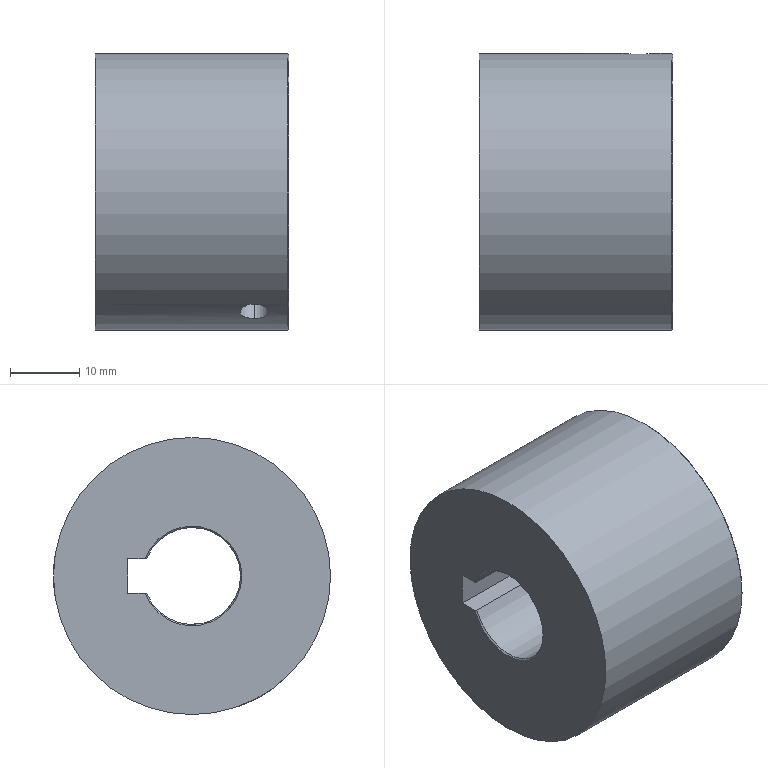Part | STEP file | ATP40XL050-B-N14 | 1 solid | 18 faces | box 28 x 40 x 40 mm | volume 30210 mm3 | cylinder 7 | cone 6 | plane 5 | commonest cylinder face diameters 4.134 x4 14 x2 40 x1
STEP:
#1=CARTESIAN_POINT('',(0.,9.3,2.5));
#2=VERTEX_POINT('',#1);
#3=CARTESIAN_POINT('',(0.,6.752,2.5));
#4=VERTEX_POINT('',#3);
#5=CARTESIAN_POINT('',(0.,9.,2.5));
#6=DIRECTION('',(0.,-1.,0.));
#7=VECTOR('',#6,1000.);
#8=LINE('',#5,#7);
#9=EDGE_CURVE('',#2,#4,#8,.T.);
#10=ORIENTED_EDGE('',*,*,#9,.T.);
#11=CARTESIAN_POINT('',(0.,-7.2,0.));
#12=VERTEX_POINT('',#11);
#13=CARTESIAN_POINT('',(0.,0.,0.));
#14=DIRECTION('',(-1.,0.,0.));
#15=DIRECTION('',(0.,1.,0.));
#16=AXIS2_PLACEMENT_3D('',#13,#14,#15);
#17=CIRCLE('',#16,7.2);
#18=EDGE_CURVE('',#12,#4,#17,.T.);
#19=ORIENTED_EDGE('',*,*,#18,.F.);
#20=CARTESIAN_POINT('',(0.,6.752,-2.5));
#21=VERTEX_POINT('',#20);
#22=CARTESIAN_POINT('',(0.,0.,0.));
#23=DIRECTION('',(-1.,0.,0.));
#24=DIRECTION('',(0.,1.,0.));
#25=AXIS2_PLACEMENT_3D('',#22,#23,#24);
#26=CIRCLE('',#25,7.2);
#27=EDGE_CURVE('',#21,#12,#26,.T.);
#28=ORIENTED_EDGE('',*,*,#27,.F.);
#29=CARTESIAN_POINT('',(0.,9.3,-2.5));
#30=VERTEX_POINT('',#29);
#31=CARTESIAN_POINT('',(0.,13.65,-2.5));
#32=DIRECTION('',(0.,1.,0.));
#33=VECTOR('',#32,1000.);
#34=LINE('',#31,#33);
#35=EDGE_CURVE('',#21,#30,#34,.T.);
#36=ORIENTED_EDGE('',*,*,#35,.T.);
#37=CARTESIAN_POINT('',(0.,9.3,1.25));
#38=DIRECTION('',(0.,0.,1.));
#39=VECTOR('',#38,1000.);
#40=LINE('',#37,#39);
#41=EDGE_CURVE('',#30,#2,#40,.T.);
#42=ORIENTED_EDGE('',*,*,#41,.T.);
#43=EDGE_LOOP('',(#10,#19,#28,#36,#42));
#44=FACE_BOUND('',#43,.T.);
#45=CARTESIAN_POINT('',(0.,0.,20.));
#46=VERTEX_POINT('',#45);
#47=CARTESIAN_POINT('',(0.,0.,0.));
#48=DIRECTION('',(-1.,0.,0.));
#49=DIRECTION('',(0.,0.,1.));
#50=AXIS2_PLACEMENT_3D('',#47,#48,#49);
#51=CIRCLE('',#50,20.);
#52=EDGE_CURVE('',#46,#46,#51,.T.);
#53=ORIENTED_EDGE('',*,*,#52,.T.);
#54=EDGE_LOOP('',(#53));
#55=FACE_OUTER_BOUND('',#54,.T.);
#56=CARTESIAN_POINT('',(0.,18.,0.));
#57=DIRECTION('',(-1.,0.,0.));
#58=DIRECTION('',(0.,0.,1.));
#59=AXIS2_PLACEMENT_3D('',#56,#57,#58);
#60=PLANE('',#59);
#61=ADVANCED_FACE('',(#44,#55),#60,.T.);
#62=CARTESIAN_POINT('',(28.,19.8,0.));
#63=VERTEX_POINT('',#62);
#64=CARTESIAN_POINT('',(27.8,20.,0.));
#65=VERTEX_POINT('',#64);
#66=CARTESIAN_POINT('',(27.9,19.9,0.));
#67=DIRECTION('',(-0.7071,0.7071,0.));
#68=VECTOR('',#67,1000.);
#69=LINE('',#66,#68);
#70=EDGE_CURVE('',#63,#65,#69,.T.);
#71=ORIENTED_EDGE('',*,*,#70,.F.);
#72=CARTESIAN_POINT('',(28.,-19.8,0.));
#73=VERTEX_POINT('',#72);
#74=CARTESIAN_POINT('',(28.,0.,0.));
#75=DIRECTION('',(-1.,0.,0.));
#76=DIRECTION('',(0.,1.,0.));
#77=AXIS2_PLACEMENT_3D('',#74,#75,#76);
#78=CIRCLE('',#77,19.8);
#79=EDGE_CURVE('',#63,#73,#78,.T.);
#80=ORIENTED_EDGE('',*,*,#79,.T.);
#81=CARTESIAN_POINT('',(27.8,-20.,0.));
#82=VERTEX_POINT('',#81);
#83=CARTESIAN_POINT('',(27.9,-19.9,0.));
#84=DIRECTION('',(0.7071,0.7071,0.));
#85=VECTOR('',#84,1000.);
#86=LINE('',#83,#85);
#87=EDGE_CURVE('',#82,#73,#86,.T.);
#88=ORIENTED_EDGE('',*,*,#87,.F.);
#89=CARTESIAN_POINT('',(27.8,0.,0.));
#90=DIRECTION('',(-1.,0.,0.));
#91=DIRECTION('',(0.,1.,0.));
#92=AXIS2_PLACEMENT_3D('',#89,#90,#91);
#93=CIRCLE('',#92,20.);
#94=EDGE_CURVE('',#65,#82,#93,.T.);
#95=ORIENTED_EDGE('',*,*,#94,.F.);
#96=EDGE_LOOP('',(#71,#80,#88,#95));
#97=FACE_OUTER_BOUND('',#96,.T.);
#98=CARTESIAN_POINT('',(27.9,0.,0.));
#99=DIRECTION('',(-1.,0.,0.));
#100=DIRECTION('',(0.,1.,0.));
#101=AXIS2_PLACEMENT_3D('',#98,#99,#100);
#102=CONICAL_SURFACE('',#101,19.9,0.7854);
#103=ADVANCED_FACE('',(#97),#102,.T.);
#104=CARTESIAN_POINT('',(0.2,-7.,0.));
#105=VERTEX_POINT('',#104);
#106=CARTESIAN_POINT('',(27.8,-7.,0.));
#107=VERTEX_POINT('',#106);
#108=CARTESIAN_POINT('',(14.,-7.,0.));
#109=DIRECTION('',(1.,0.,0.));
#110=VECTOR('',#109,1000.);
#111=LINE('',#108,#110);
#112=EDGE_CURVE('',#105,#107,#111,.T.);
#113=ORIENTED_EDGE('',*,*,#112,.F.);
#114=CARTESIAN_POINT('',(0.2,6.538,2.5));
#115=VERTEX_POINT('',#114);
#116=CARTESIAN_POINT('',(0.2,0.,0.));
#117=DIRECTION('',(-1.,0.,0.));
#118=DIRECTION('',(0.,1.,0.));
#119=AXIS2_PLACEMENT_3D('',#116,#117,#118);
#120=CIRCLE('',#119,7.);
#121=EDGE_CURVE('',#105,#115,#120,.T.);
#122=ORIENTED_EDGE('',*,*,#121,.T.);
#123=CARTESIAN_POINT('',(27.8,6.538,2.5));
#124=VERTEX_POINT('',#123);
#125=CARTESIAN_POINT('',(14.,6.538,2.5));
#126=DIRECTION('',(1.,0.,0.));
#127=VECTOR('',#126,1000.);
#128=LINE('',#125,#127);
#129=EDGE_CURVE('',#115,#124,#128,.T.);
#130=ORIENTED_EDGE('',*,*,#129,.T.);
#131=CARTESIAN_POINT('',(27.8,0.,0.));
#132=DIRECTION('',(-1.,0.,0.));
#133=DIRECTION('',(0.,1.,0.));
#134=AXIS2_PLACEMENT_3D('',#131,#132,#133);
#135=CIRCLE('',#134,7.);
#136=EDGE_CURVE('',#107,#124,#135,.T.);
#137=ORIENTED_EDGE('',*,*,#136,.F.);
#138=EDGE_LOOP('',(#113,#122,#130,#137));
#139=FACE_OUTER_BOUND('',#138,.T.);
#140=CARTESIAN_POINT('',(14.,0.,0.));
#141=DIRECTION('',(1.,0.,0.));
#142=DIRECTION('',(0.,1.,0.));
#143=AXIS2_PLACEMENT_3D('',#140,#141,#142);
#144=CYLINDRICAL_SURFACE('',#143,7.);
#145=ADVANCED_FACE('',(#139),#144,.F.);
#146=CARTESIAN_POINT('',(0.1,-7.1,0.));
#147=DIRECTION('',(0.7071,0.7071,0.));
#148=VECTOR('',#147,1000.);
#149=LINE('',#146,#148);
#150=EDGE_CURVE('',#12,#105,#149,.T.);
#151=ORIENTED_EDGE('',*,*,#150,.F.);
#152=ORIENTED_EDGE('',*,*,#18,.T.);
#153=CARTESIAN_POINT('',(0.,6.752,2.5));
#154=CARTESIAN_POINT('',(0.1016,6.644,2.5));
#155=CARTESIAN_POINT('',(0.2,6.538,2.5));
#156=(BOUNDED_CURVE()B_SPLINE_CURVE(2,(#153,#154,#155),.UNSPECIFIED.,.F.,.F.)B_SPLINE_CURVE_WITH_KNOTS((3,3),(0.,0.2927),.UNSPECIFIED.)CURVE()GEOMETRIC_REPRESENTATION_ITEM()RATIONAL_B_SPLINE_CURVE((1.,1.,1.))REPRESENTATION_ITEM(''));
#157=EDGE_CURVE('',#4,#115,#156,.T.);
#158=ORIENTED_EDGE('',*,*,#157,.T.);
#159=ORIENTED_EDGE('',*,*,#121,.F.);
#160=EDGE_LOOP('',(#151,#152,#158,#159));
#161=FACE_OUTER_BOUND('',#160,.T.);
#162=CARTESIAN_POINT('',(0.1,0.,0.));
#163=DIRECTION('',(-1.,0.,0.));
#164=DIRECTION('',(0.,1.,0.));
#165=AXIS2_PLACEMENT_3D('',#162,#163,#164);
#166=CONICAL_SURFACE('',#165,7.1,0.7854);
#167=ADVANCED_FACE('',(#161),#166,.F.);
#168=CARTESIAN_POINT('',(28.,-7.2,0.));
#169=VERTEX_POINT('',#168);
#170=CARTESIAN_POINT('',(27.9,-7.1,0.));
#171=DIRECTION('',(0.7071,-0.7071,0.));
#172=VECTOR('',#171,1000.);
#173=LINE('',#170,#172);
#174=EDGE_CURVE('',#107,#169,#173,.T.);
#175=ORIENTED_EDGE('',*,*,#174,.F.);
#176=ORIENTED_EDGE('',*,*,#136,.T.);
#177=CARTESIAN_POINT('',(28.,6.752,2.5));
#178=VERTEX_POINT('',#177);
#179=CARTESIAN_POINT('',(27.8,6.538,2.5));
#180=CARTESIAN_POINT('',(27.898,6.644,2.5));
#181=CARTESIAN_POINT('',(28.,6.752,2.5));
#182=(BOUNDED_CURVE()B_SPLINE_CURVE(2,(#179,#180,#181),.UNSPECIFIED.,.F.,.T.)B_SPLINE_CURVE_WITH_KNOTS((3,3),(0.,0.2927),.UNSPECIFIED.)CURVE()GEOMETRIC_REPRESENTATION_ITEM()RATIONAL_B_SPLINE_CURVE((1.,1.,1.))REPRESENTATION_ITEM(''));
#183=EDGE_CURVE('',#124,#178,#182,.T.);
#184=ORIENTED_EDGE('',*,*,#183,.T.);
#185=CARTESIAN_POINT('',(28.,0.,0.));
#186=DIRECTION('',(-1.,0.,0.));
#187=DIRECTION('',(0.,1.,0.));
#188=AXIS2_PLACEMENT_3D('',#185,#186,#187);
#189=CIRCLE('',#188,7.2);
#190=EDGE_CURVE('',#169,#178,#189,.T.);
#191=ORIENTED_EDGE('',*,*,#190,.F.);
#192=EDGE_LOOP('',(#175,#176,#184,#191));
#193=FACE_OUTER_BOUND('',#192,.T.);
#194=CARTESIAN_POINT('',(27.9,0.,0.));
#195=DIRECTION('',(1.,0.,0.));
#196=DIRECTION('',(0.,1.,0.));
#197=AXIS2_PLACEMENT_3D('',#194,#195,#196);
#198=CONICAL_SURFACE('',#197,7.1,0.7854);
#199=ADVANCED_FACE('',(#193),#198,.F.);
#200=CARTESIAN_POINT('',(23.,19.893,-2.067));
#201=VERTEX_POINT('',#200);
#202=CARTESIAN_POINT('',(23.,19.893,2.067));
#203=VERTEX_POINT('',#202);
#204=CARTESIAN_POINT('',(23.,19.893,-2.067));
#205=CARTESIAN_POINT('',(23.137,19.893,-2.067));
#206=CARTESIAN_POINT('',(23.271,19.894,-2.054));
#207=CARTESIAN_POINT('',(23.535,19.9,-2.001));
#208=CARTESIAN_POINT('',(23.666,19.904,-1.961));
#209=CARTESIAN_POINT('',(23.916,19.914,-1.858));
#210=CARTESIAN_POINT('',(24.035,19.919,-1.794));
#211=CARTESIAN_POINT('',(24.26,19.932,-1.644));
#212=CARTESIAN_POINT('',(24.366,19.94,-1.557));
#213=CARTESIAN_POINT('',(24.652,19.96,-1.272));
#214=CARTESIAN_POINT('',(24.806,19.974,-1.041));
#215=CARTESIAN_POINT('',(25.012,19.994,-0.5445));
#216=CARTESIAN_POINT('',(25.067,20.,-0.2731));
#217=CARTESIAN_POINT('',(25.067,20.,0.1366));
#218=CARTESIAN_POINT('',(25.054,19.999,0.2709));
#219=CARTESIAN_POINT('',(25.001,19.993,0.535));
#220=CARTESIAN_POINT('',(24.961,19.989,0.6663));
#221=CARTESIAN_POINT('',(24.858,19.979,0.9164));
#222=CARTESIAN_POINT('',(24.794,19.974,1.035));
#223=CARTESIAN_POINT('',(24.644,19.961,1.26));
#224=CARTESIAN_POINT('',(24.557,19.954,1.366));
#225=CARTESIAN_POINT('',(24.272,19.933,1.652));
#226=CARTESIAN_POINT('',(24.041,19.919,1.806));
#227=CARTESIAN_POINT('',(23.545,19.899,2.012));
#228=CARTESIAN_POINT('',(23.273,19.893,2.067));
#229=CARTESIAN_POINT('',(23.,19.893,2.067));
#230=B_SPLINE_CURVE_WITH_KNOTS('',3,(#204,#205,#206,#207,#208,#209,#210,#211,#212,#213,#214,#215,#216,#217,#218,#219,#220,#221,#222,#223,#224,#225,#226,#227,#228,#229),.UNSPECIFIED.,.F.,.F.,(4,2,2,2,2,2,2,2,2,2,2,2,4),(0.,0.0004039,0.0008078,0.001212,0.001616,0.002423,0.003231,0.003635,0.004039,0.004443,0.004847,0.005655,0.006462),.UNSPECIFIED.);
#231=EDGE_CURVE('',#201,#203,#230,.T.);
#232=ORIENTED_EDGE('',*,*,#231,.T.);
#233=CARTESIAN_POINT('',(23.,19.893,2.067));
#234=CARTESIAN_POINT('',(22.863,19.893,2.067));
#235=CARTESIAN_POINT('',(22.729,19.894,2.054));
#236=CARTESIAN_POINT('',(22.465,19.9,2.001));
#237=CARTESIAN_POINT('',(22.334,19.904,1.961));
#238=CARTESIAN_POINT('',(22.084,19.914,1.858));
#239=CARTESIAN_POINT('',(21.965,19.919,1.794));
#240=CARTESIAN_POINT('',(21.74,19.932,1.644));
#241=CARTESIAN_POINT('',(21.634,19.94,1.557));
#242=CARTESIAN_POINT('',(21.348,19.96,1.272));
#243=CARTESIAN_POINT('',(21.194,19.974,1.041));
#244=CARTESIAN_POINT('',(20.988,19.994,0.5445));
#245=CARTESIAN_POINT('',(20.933,20.,0.2731));
#246=CARTESIAN_POINT('',(20.933,20.,-0.1366));
#247=CARTESIAN_POINT('',(20.946,19.999,-0.2709));
#248=CARTESIAN_POINT('',(20.999,19.993,-0.535));
#249=CARTESIAN_POINT('',(21.039,19.989,-0.6663));
#250=CARTESIAN_POINT('',(21.142,19.979,-0.9164));
#251=CARTESIAN_POINT('',(21.206,19.974,-1.035));
#252=CARTESIAN_POINT('',(21.356,19.961,-1.26));
#253=CARTESIAN_POINT('',(21.443,19.954,-1.366));
#254=CARTESIAN_POINT('',(21.728,19.933,-1.652));
#255=CARTESIAN_POINT('',(21.959,19.919,-1.806));
#256=CARTESIAN_POINT('',(22.455,19.899,-2.012));
#257=CARTESIAN_POINT('',(22.727,19.893,-2.067));
#258=CARTESIAN_POINT('',(23.,19.893,-2.067));
#259=B_SPLINE_CURVE_WITH_KNOTS('',3,(#233,#234,#235,#236,#237,#238,#239,#240,#241,#242,#243,#244,#245,#246,#247,#248,#249,#250,#251,#252,#253,#254,#255,#256,#257,#258),.UNSPECIFIED.,.F.,.F.,(4,2,2,2,2,2,2,2,2,2,2,2,4),(-0.003231,-0.002827,-0.002423,-0.002019,-0.001616,-0.0008078,0.000000013,0.0004039,0.0008078,0.001212,0.001616,0.002423,0.003231),.UNSPECIFIED.);
#260=EDGE_CURVE('',#203,#201,#259,.T.);
#261=ORIENTED_EDGE('',*,*,#260,.T.);
#262=EDGE_LOOP('',(#232,#261));
#263=FACE_BOUND('',#262,.T.);
#264=ORIENTED_EDGE('',*,*,#94,.T.);
#265=CARTESIAN_POINT('',(27.8,0.,0.));
#266=DIRECTION('',(-1.,0.,0.));
#267=DIRECTION('',(0.,1.,0.));
#268=AXIS2_PLACEMENT_3D('',#265,#266,#267);
#269=CIRCLE('',#268,20.);
#270=EDGE_CURVE('',#82,#65,#269,.T.);
#271=ORIENTED_EDGE('',*,*,#270,.T.);
#272=EDGE_LOOP('',(#264,#271));
#273=FACE_OUTER_BOUND('',#272,.T.);
#274=CARTESIAN_POINT('',(23.,-11.737,-16.194));
#275=VERTEX_POINT('',#274);
#276=CARTESIAN_POINT('',(23.,-8.156,-18.261));
#277=VERTEX_POINT('',#276);
#278=CARTESIAN_POINT('',(23.,-11.737,-16.194));
#279=CARTESIAN_POINT('',(23.137,-11.737,-16.194));
#280=CARTESIAN_POINT('',(23.271,-11.726,-16.202));
#281=CARTESIAN_POINT('',(23.535,-11.683,-16.233));
#282=CARTESIAN_POINT('',(23.666,-11.65,-16.256));
#283=CARTESIAN_POINT('',(23.916,-11.566,-16.317));
#284=CARTESIAN_POINT('',(24.035,-11.514,-16.354));
#285=CARTESIAN_POINT('',(24.26,-11.39,-16.44));
#286=CARTESIAN_POINT('',(24.366,-11.318,-16.489));
#287=CARTESIAN_POINT('',(24.652,-11.082,-16.65));
#288=CARTESIAN_POINT('',(24.806,-10.889,-16.778));
#289=CARTESIAN_POINT('',(25.012,-10.469,-17.043));
#290=CARTESIAN_POINT('',(25.067,-10.237,-17.184));
#291=CARTESIAN_POINT('',(25.067,-9.882,-17.389));
#292=CARTESIAN_POINT('',(25.054,-9.765,-17.455));
#293=CARTESIAN_POINT('',(25.001,-9.533,-17.582));
#294=CARTESIAN_POINT('',(24.961,-9.418,-17.644));
#295=CARTESIAN_POINT('',(24.858,-9.196,-17.761));
#296=CARTESIAN_POINT('',(24.794,-9.09,-17.815));
#297=CARTESIAN_POINT('',(24.644,-8.889,-17.916));
#298=CARTESIAN_POINT('',(24.557,-8.794,-17.963));
#299=CARTESIAN_POINT('',(24.272,-8.536,-18.088));
#300=CARTESIAN_POINT('',(24.041,-8.396,-18.153));
#301=CARTESIAN_POINT('',(23.545,-8.207,-18.239));
#302=CARTESIAN_POINT('',(23.273,-8.156,-18.261));
#303=CARTESIAN_POINT('',(23.,-8.156,-18.261));
#304=B_SPLINE_CURVE_WITH_KNOTS('',3,(#278,#279,#280,#281,#282,#283,#284,#285,#286,#287,#288,#289,#290,#291,#292,#293,#294,#295,#296,#297,#298,#299,#300,#301,#302,#303),.UNSPECIFIED.,.F.,.F.,(4,2,2,2,2,2,2,2,2,2,2,2,4),(-0.003231,-0.002827,-0.002423,-0.002019,-0.001616,-0.0008078,0.000000013,0.0004039,0.0008078,0.001212,0.001616,0.002423,0.003231),.UNSPECIFIED.);
#305=EDGE_CURVE('',#275,#277,#304,.T.);
#306=ORIENTED_EDGE('',*,*,#305,.T.);
#307=CARTESIAN_POINT('',(23.,-8.156,-18.261));
#308=CARTESIAN_POINT('',(22.863,-8.156,-18.261));
#309=CARTESIAN_POINT('',(22.729,-8.169,-18.256));
#310=CARTESIAN_POINT('',(22.465,-8.217,-18.234));
#311=CARTESIAN_POINT('',(22.334,-8.253,-18.218));
#312=CARTESIAN_POINT('',(22.084,-8.348,-18.175));
#313=CARTESIAN_POINT('',(21.965,-8.406,-18.148));
#314=CARTESIAN_POINT('',(21.74,-8.542,-18.084));
#315=CARTESIAN_POINT('',(21.634,-8.621,-18.047));
#316=CARTESIAN_POINT('',(21.348,-8.879,-17.922));
#317=CARTESIAN_POINT('',(21.194,-9.085,-17.819));
#318=CARTESIAN_POINT('',(20.988,-9.525,-17.588));
#319=CARTESIAN_POINT('',(20.933,-9.763,-17.457));
#320=CARTESIAN_POINT('',(20.933,-10.118,-17.252));
#321=CARTESIAN_POINT('',(20.946,-10.234,-17.184));
#322=CARTESIAN_POINT('',(20.999,-10.46,-17.047));
#323=CARTESIAN_POINT('',(21.039,-10.572,-16.978));
#324=CARTESIAN_POINT('',(21.142,-10.783,-16.844));
#325=CARTESIAN_POINT('',(21.206,-10.883,-16.78));
#326=CARTESIAN_POINT('',(21.356,-11.071,-16.657));
#327=CARTESIAN_POINT('',(21.443,-11.16,-16.597));
#328=CARTESIAN_POINT('',(21.728,-11.397,-16.436));
#329=CARTESIAN_POINT('',(21.959,-11.523,-16.347));
#330=CARTESIAN_POINT('',(22.455,-11.692,-16.227));
#331=CARTESIAN_POINT('',(22.727,-11.737,-16.194));
#332=CARTESIAN_POINT('',(23.,-11.737,-16.194));
#333=B_SPLINE_CURVE_WITH_KNOTS('',3,(#307,#308,#309,#310,#311,#312,#313,#314,#315,#316,#317,#318,#319,#320,#321,#322,#323,#324,#325,#326,#327,#328,#329,#330,#331,#332),.UNSPECIFIED.,.F.,.F.,(4,2,2,2,2,2,2,2,2,2,2,2,4),(0.,0.0004039,0.0008078,0.001212,0.001616,0.002423,0.003231,0.003635,0.004039,0.004443,0.004847,0.005655,0.006462),.UNSPECIFIED.);
#334=EDGE_CURVE('',#277,#275,#333,.T.);
#335=ORIENTED_EDGE('',*,*,#334,.T.);
#336=EDGE_LOOP('',(#306,#335));
#337=FACE_BOUND('',#336,.T.);
#338=ORIENTED_EDGE('',*,*,#52,.F.);
#339=EDGE_LOOP('',(#338));
#340=FACE_OUTER_BOUND('',#339,.T.);
#341=CARTESIAN_POINT('',(23.4,0.,0.));
#342=DIRECTION('',(1.,0.,0.));
#343=DIRECTION('',(0.,1.,0.));
#344=AXIS2_PLACEMENT_3D('',#341,#342,#343);
#345=CYLINDRICAL_SURFACE('',#344,20.);
#346=ADVANCED_FACE('',(#263,#273,#337,#340),#345,.T.);
#347=CARTESIAN_POINT('',(23.,9.3,2.067));
#348=VERTEX_POINT('',#347);
#349=CARTESIAN_POINT('',(23.,14.65,2.067));
#350=DIRECTION('',(0.,1.,0.));
#351=VECTOR('',#350,1000.);
#352=LINE('',#349,#351);
#353=EDGE_CURVE('',#348,#203,#352,.T.);
#354=ORIENTED_EDGE('',*,*,#353,.F.);
#355=CARTESIAN_POINT('',(23.,9.3,-2.067));
#356=VERTEX_POINT('',#355);
#357=CARTESIAN_POINT('',(23.,9.3,0.));
#358=DIRECTION('',(0.,1.,0.));
#359=DIRECTION('',(0.,0.,1.));
#360=AXIS2_PLACEMENT_3D('',#357,#358,#359);
#361=CIRCLE('',#360,2.067);
#362=EDGE_CURVE('',#356,#348,#361,.T.);
#363=ORIENTED_EDGE('',*,*,#362,.F.);
#364=CARTESIAN_POINT('',(23.,14.65,-2.067));
#365=DIRECTION('',(0.,-1.,0.));
#366=VECTOR('',#365,1000.);
#367=LINE('',#364,#366);
#368=EDGE_CURVE('',#201,#356,#367,.T.);
#369=ORIENTED_EDGE('',*,*,#368,.F.);
#370=ORIENTED_EDGE('',*,*,#260,.F.);
#371=EDGE_LOOP('',(#354,#363,#369,#370));
#372=FACE_OUTER_BOUND('',#371,.T.);
#373=CARTESIAN_POINT('',(23.,14.65,0.));
#374=DIRECTION('',(0.,1.,0.));
#375=DIRECTION('',(0.,0.,1.));
#376=AXIS2_PLACEMENT_3D('',#373,#374,#375);
#377=CYLINDRICAL_SURFACE('',#376,2.067);
#378=ADVANCED_FACE('',(#372),#377,.F.);
#379=CARTESIAN_POINT('',(23.,-5.134,-4.758));
#380=VERTEX_POINT('',#379);
#381=CARTESIAN_POINT('',(23.,-8.29,-10.225));
#382=DIRECTION('',(0.,0.5,0.866));
#383=VECTOR('',#382,1000.);
#384=LINE('',#381,#383);
#385=EDGE_CURVE('',#275,#380,#384,.T.);
#386=ORIENTED_EDGE('',*,*,#385,.F.);
#387=ORIENTED_EDGE('',*,*,#334,.F.);
#388=CARTESIAN_POINT('',(23.,-1.554,-6.825));
#389=VERTEX_POINT('',#388);
#390=CARTESIAN_POINT('',(23.,-4.71,-12.292));
#391=DIRECTION('',(0.,-0.5,-0.866));
#392=VECTOR('',#391,1000.);
#393=LINE('',#390,#392);
#394=EDGE_CURVE('',#389,#277,#393,.T.);
#395=ORIENTED_EDGE('',*,*,#394,.F.);
#396=CARTESIAN_POINT('',(23.,-5.134,-4.758));
#397=CARTESIAN_POINT('',(22.726,-5.134,-4.758));
#398=CARTESIAN_POINT('',(22.46,-5.097,-4.8));
#399=CARTESIAN_POINT('',(22.144,-5.001,-4.898));
#400=CARTESIAN_POINT('',(22.082,-4.98,-4.919));
#401=CARTESIAN_POINT('',(21.992,-4.945,-4.955));
#402=CARTESIAN_POINT('',(21.962,-4.932,-4.967));
#403=CARTESIAN_POINT('',(21.903,-4.906,-4.993));
#404=CARTESIAN_POINT('',(21.873,-4.892,-5.007));
#405=CARTESIAN_POINT('',(21.735,-4.823,-5.074));
#406=CARTESIAN_POINT('',(21.633,-4.76,-5.133));
#407=CARTESIAN_POINT('',(21.492,-4.653,-5.23));
#408=CARTESIAN_POINT('',(21.447,-4.615,-5.263));
#409=CARTESIAN_POINT('',(21.363,-4.537,-5.331));
#410=CARTESIAN_POINT('',(21.324,-4.497,-5.365));
#411=CARTESIAN_POINT('',(21.209,-4.363,-5.475));
#412=CARTESIAN_POINT('',(21.144,-4.267,-5.55));
#413=CARTESIAN_POINT('',(20.986,-3.959,-5.778));
#414=CARTESIAN_POINT('',(20.933,-3.738,-5.925));
#415=CARTESIAN_POINT('',(20.933,-3.262,-6.199));
#416=CARTESIAN_POINT('',(20.986,-3.025,-6.318));
#417=CARTESIAN_POINT('',(21.118,-2.732,-6.445));
#418=CARTESIAN_POINT('',(21.147,-2.674,-6.469));
#419=CARTESIAN_POINT('',(21.212,-2.562,-6.515));
#420=CARTESIAN_POINT('',(21.248,-2.505,-6.537));
#421=CARTESIAN_POINT('',(21.36,-2.347,-6.596));
#422=CARTESIAN_POINT('',(21.444,-2.249,-6.63));
#423=CARTESIAN_POINT('',(21.586,-2.111,-6.674));
#424=CARTESIAN_POINT('',(21.66,-2.046,-6.695));
#425=CARTESIAN_POINT('',(21.738,-1.985,-6.713));
#426=CARTESIAN_POINT('',(21.791,-1.946,-6.724));
#427=CARTESIAN_POINT('',(21.817,-1.928,-6.729));
#428=CARTESIAN_POINT('',(21.96,-1.832,-6.756));
#429=CARTESIAN_POINT('',(22.08,-1.768,-6.773));
#430=CARTESIAN_POINT('',(22.461,-1.608,-6.814));
#431=CARTESIAN_POINT('',(22.726,-1.554,-6.825));
#432=CARTESIAN_POINT('',(23.,-1.554,-6.825));
#433=B_SPLINE_CURVE_WITH_KNOTS('',3,(#396,#397,#398,#399,#400,#401,#402,#403,#404,#405,#406,#407,#408,#409,#410,#411,#412,#413,#414,#415,#416,#417,#418,#419,#420,#421,#422,#423,#424,#425,#426,#427,#428,#429,#430,#431,#432),.UNSPECIFIED.,.F.,.F.,(4,2,2,2,2,2,2,2,2,2,2,2,2,2,1,2,2,2,4),(0.,0.125,0.1563,0.1719,0.1875,0.25,0.2812,0.3125,0.375,0.5,0.625,0.6562,0.6875,0.75,0.7812,0.7969,0.8125,0.875,1.),.UNSPECIFIED.);
#434=EDGE_CURVE('',#380,#389,#433,.T.);
#435=ORIENTED_EDGE('',*,*,#434,.F.);
#436=EDGE_LOOP('',(#386,#387,#395,#435));
#437=FACE_OUTER_BOUND('',#436,.T.);
#438=CARTESIAN_POINT('',(23.,-6.5,-11.258));
#439=DIRECTION('',(0.,0.5,0.866));
#440=DIRECTION('',(0.,-0.866,0.5));
#441=AXIS2_PLACEMENT_3D('',#438,#439,#440);
#442=CYLINDRICAL_SURFACE('',#441,2.067);
#443=ADVANCED_FACE('',(#437),#442,.F.);
#444=ORIENTED_EDGE('',*,*,#385,.T.);
#445=CARTESIAN_POINT('',(23.,-1.554,-6.825));
#446=CARTESIAN_POINT('',(23.274,-1.554,-6.825));
#447=CARTESIAN_POINT('',(23.54,-1.608,-6.814));
#448=CARTESIAN_POINT('',(23.856,-1.741,-6.78));
#449=CARTESIAN_POINT('',(23.918,-1.77,-6.773));
#450=CARTESIAN_POINT('',(24.008,-1.819,-6.76));
#451=CARTESIAN_POINT('',(24.038,-1.836,-6.755));
#452=CARTESIAN_POINT('',(24.097,-1.871,-6.745));
#453=CARTESIAN_POINT('',(24.127,-1.89,-6.74));
#454=CARTESIAN_POINT('',(24.265,-1.982,-6.714));
#455=CARTESIAN_POINT('',(24.367,-2.065,-6.689));
#456=CARTESIAN_POINT('',(24.508,-2.203,-6.645));
#457=CARTESIAN_POINT('',(24.553,-2.25,-6.629));
#458=CARTESIAN_POINT('',(24.637,-2.349,-6.594));
#459=CARTESIAN_POINT('',(24.676,-2.398,-6.577));
#460=CARTESIAN_POINT('',(24.791,-2.56,-6.516));
#461=CARTESIAN_POINT('',(24.856,-2.673,-6.471));
#462=CARTESIAN_POINT('',(25.014,-3.025,-6.318));
#463=CARTESIAN_POINT('',(25.067,-3.262,-6.199));
#464=CARTESIAN_POINT('',(25.067,-3.738,-5.925));
#465=CARTESIAN_POINT('',(25.014,-3.959,-5.778));
#466=CARTESIAN_POINT('',(24.882,-4.216,-5.588));
#467=CARTESIAN_POINT('',(24.853,-4.265,-5.551));
#468=CARTESIAN_POINT('',(24.788,-4.361,-5.476));
#469=CARTESIAN_POINT('',(24.752,-4.409,-5.437));
#470=CARTESIAN_POINT('',(24.64,-4.539,-5.33));
#471=CARTESIAN_POINT('',(24.556,-4.617,-5.262));
#472=CARTESIAN_POINT('',(24.414,-4.725,-5.165));
#473=CARTESIAN_POINT('',(24.365,-4.758,-5.134));
#474=CARTESIAN_POINT('',(24.288,-4.806,-5.09));
#475=CARTESIAN_POINT('',(24.262,-4.821,-5.075));
#476=CARTESIAN_POINT('',(24.209,-4.85,-5.047));
#477=CARTESIAN_POINT('',(24.183,-4.864,-5.034));
#478=CARTESIAN_POINT('',(24.04,-4.935,-4.965));
#479=CARTESIAN_POINT('',(23.92,-4.982,-4.917));
#480=CARTESIAN_POINT('',(23.539,-5.097,-4.799));
#481=CARTESIAN_POINT('',(23.274,-5.134,-4.758));
#482=CARTESIAN_POINT('',(23.,-5.134,-4.758));
#483=B_SPLINE_CURVE_WITH_KNOTS('',3,(#445,#446,#447,#448,#449,#450,#451,#452,#453,#454,#455,#456,#457,#458,#459,#460,#461,#462,#463,#464,#465,#466,#467,#468,#469,#470,#471,#472,#473,#474,#475,#476,#477,#478,#479,#480,#481,#482),.UNSPECIFIED.,.F.,.F.,(4,2,2,2,2,2,2,2,2,2,2,2,2,2,2,2,2,2,4),(0.,0.125,0.1562,0.1719,0.1875,0.25,0.2812,0.3125,0.375,0.5,0.625,0.6562,0.6875,0.75,0.7812,0.7969,0.8125,0.875,1.),.UNSPECIFIED.);
#484=EDGE_CURVE('',#389,#380,#483,.T.);
#485=ORIENTED_EDGE('',*,*,#484,.F.);
#486=ORIENTED_EDGE('',*,*,#394,.T.);
#487=ORIENTED_EDGE('',*,*,#305,.F.);
#488=EDGE_LOOP('',(#444,#485,#486,#487));
#489=FACE_OUTER_BOUND('',#488,.T.);
#490=CARTESIAN_POINT('',(23.,-6.5,-11.258));
#491=DIRECTION('',(0.,0.5,0.866));
#492=DIRECTION('',(0.,-0.866,0.5));
#493=AXIS2_PLACEMENT_3D('',#490,#491,#492);
#494=CYLINDRICAL_SURFACE('',#493,2.067);
#495=ADVANCED_FACE('',(#489),#494,.F.);
#496=ORIENTED_EDGE('',*,*,#353,.T.);
#497=ORIENTED_EDGE('',*,*,#231,.F.);
#498=ORIENTED_EDGE('',*,*,#368,.T.);
#499=CARTESIAN_POINT('',(23.,9.3,0.));
#500=DIRECTION('',(0.,1.,0.));
#501=DIRECTION('',(0.,0.,1.));
#502=AXIS2_PLACEMENT_3D('',#499,#500,#501);
#503=CIRCLE('',#502,2.067);
#504=EDGE_CURVE('',#348,#356,#503,.T.);
#505=ORIENTED_EDGE('',*,*,#504,.F.);
#506=EDGE_LOOP('',(#496,#497,#498,#505));
#507=FACE_OUTER_BOUND('',#506,.T.);
#508=CARTESIAN_POINT('',(23.,14.65,0.));
#509=DIRECTION('',(0.,1.,0.));
#510=DIRECTION('',(0.,0.,1.));
#511=AXIS2_PLACEMENT_3D('',#508,#509,#510);
#512=CYLINDRICAL_SURFACE('',#511,2.067);
#513=ADVANCED_FACE('',(#507),#512,.F.);
#514=CARTESIAN_POINT('',(28.,6.752,-2.5));
#515=VERTEX_POINT('',#514);
#516=CARTESIAN_POINT('',(27.8,6.538,-2.5));
#517=VERTEX_POINT('',#516);
#518=CARTESIAN_POINT('',(28.,6.752,-2.5));
#519=CARTESIAN_POINT('',(27.898,6.644,-2.5));
#520=CARTESIAN_POINT('',(27.8,6.538,-2.5));
#521=(BOUNDED_CURVE()B_SPLINE_CURVE(2,(#518,#519,#520),.UNSPECIFIED.,.F.,.F.)B_SPLINE_CURVE_WITH_KNOTS((3,3),(0.,0.2927),.UNSPECIFIED.)CURVE()GEOMETRIC_REPRESENTATION_ITEM()RATIONAL_B_SPLINE_CURVE((1.,1.,1.))REPRESENTATION_ITEM(''));
#522=EDGE_CURVE('',#515,#517,#521,.T.);
#523=ORIENTED_EDGE('',*,*,#522,.F.);
#524=CARTESIAN_POINT('',(28.,9.3,-2.5));
#525=VERTEX_POINT('',#524);
#526=CARTESIAN_POINT('',(28.,11.4,-2.5));
#527=DIRECTION('',(0.,-1.,0.));
#528=VECTOR('',#527,1000.);
#529=LINE('',#526,#528);
#530=EDGE_CURVE('',#525,#515,#529,.T.);
#531=ORIENTED_EDGE('',*,*,#530,.F.);
#532=CARTESIAN_POINT('',(0.,9.3,-2.5));
#533=DIRECTION('',(1.,0.,0.));
#534=VECTOR('',#533,1000.);
#535=LINE('',#532,#534);
#536=EDGE_CURVE('',#30,#525,#535,.T.);
#537=ORIENTED_EDGE('',*,*,#536,.F.);
#538=ORIENTED_EDGE('',*,*,#35,.F.);
#539=CARTESIAN_POINT('',(0.2,6.538,-2.5));
#540=VERTEX_POINT('',#539);
#541=CARTESIAN_POINT('',(0.2,6.538,-2.5));
#542=CARTESIAN_POINT('',(0.1016,6.644,-2.5));
#543=CARTESIAN_POINT('',(0.,6.752,-2.5));
#544=(BOUNDED_CURVE()B_SPLINE_CURVE(2,(#541,#542,#543),.UNSPECIFIED.,.F.,.F.)B_SPLINE_CURVE_WITH_KNOTS((3,3),(0.,0.2927),.UNSPECIFIED.)CURVE()GEOMETRIC_REPRESENTATION_ITEM()RATIONAL_B_SPLINE_CURVE((1.,1.,1.))REPRESENTATION_ITEM(''));
#545=EDGE_CURVE('',#540,#21,#544,.T.);
#546=ORIENTED_EDGE('',*,*,#545,.F.);
#547=CARTESIAN_POINT('',(14.,6.538,-2.5));
#548=DIRECTION('',(-1.,0.,0.));
#549=VECTOR('',#548,1000.);
#550=LINE('',#547,#549);
#551=EDGE_CURVE('',#517,#540,#550,.T.);
#552=ORIENTED_EDGE('',*,*,#551,.F.);
#553=EDGE_LOOP('',(#523,#531,#537,#538,#546,#552));
#554=FACE_OUTER_BOUND('',#553,.T.);
#555=CARTESIAN_POINT('',(0.,9.3,-2.5));
#556=DIRECTION('',(0.,0.,-1.));
#557=DIRECTION('',(0.,-1.,0.));
#558=AXIS2_PLACEMENT_3D('',#555,#556,#557);
#559=PLANE('',#558);
#560=ADVANCED_FACE('',(#554),#559,.F.);
#561=ORIENTED_EDGE('',*,*,#183,.F.);
#562=ORIENTED_EDGE('',*,*,#129,.F.);
#563=ORIENTED_EDGE('',*,*,#157,.F.);
#564=ORIENTED_EDGE('',*,*,#9,.F.);
#565=CARTESIAN_POINT('',(28.,9.3,2.5));
#566=VERTEX_POINT('',#565);
#567=CARTESIAN_POINT('',(0.,9.3,2.5));
#568=DIRECTION('',(1.,0.,0.));
#569=VECTOR('',#568,1000.);
#570=LINE('',#567,#569);
#571=EDGE_CURVE('',#2,#566,#570,.T.);
#572=ORIENTED_EDGE('',*,*,#571,.T.);
#573=CARTESIAN_POINT('',(28.,6.75,2.5));
#574=DIRECTION('',(0.,1.,0.));
#575=VECTOR('',#574,1000.);
#576=LINE('',#573,#575);
#577=EDGE_CURVE('',#178,#566,#576,.T.);
#578=ORIENTED_EDGE('',*,*,#577,.F.);
#579=EDGE_LOOP('',(#561,#562,#563,#564,#572,#578));
#580=FACE_OUTER_BOUND('',#579,.T.);
#581=CARTESIAN_POINT('',(0.,0.,2.5));
#582=DIRECTION('',(0.,0.,1.));
#583=DIRECTION('',(1.,0.,0.));
#584=AXIS2_PLACEMENT_3D('',#581,#582,#583);
#585=PLANE('',#584);
#586=ADVANCED_FACE('',(#580),#585,.F.);
#587=CARTESIAN_POINT('',(28.,9.3,1.25));
#588=DIRECTION('',(0.,0.,-1.));
#589=VECTOR('',#588,1000.);
#590=LINE('',#587,#589);
#591=EDGE_CURVE('',#566,#525,#590,.T.);
#592=ORIENTED_EDGE('',*,*,#591,.F.);
#593=ORIENTED_EDGE('',*,*,#571,.F.);
#594=ORIENTED_EDGE('',*,*,#41,.F.);
#595=ORIENTED_EDGE('',*,*,#536,.T.);
#596=EDGE_LOOP('',(#592,#593,#594,#595));
#597=FACE_OUTER_BOUND('',#596,.T.);
#598=ORIENTED_EDGE('',*,*,#504,.T.);
#599=ORIENTED_EDGE('',*,*,#362,.T.);
#600=EDGE_LOOP('',(#598,#599));
#601=FACE_BOUND('',#600,.T.);
#602=CARTESIAN_POINT('',(0.,9.3,2.5));
#603=DIRECTION('',(0.,1.,0.));
#604=DIRECTION('',(1.,0.,0.));
#605=AXIS2_PLACEMENT_3D('',#602,#603,#604);
#606=PLANE('',#605);
#607=ADVANCED_FACE('',(#597,#601),#606,.F.);
#608=ORIENTED_EDGE('',*,*,#79,.F.);
#609=CARTESIAN_POINT('',(28.,0.,0.));
#610=DIRECTION('',(-1.,0.,0.));
#611=DIRECTION('',(0.,1.,0.));
#612=AXIS2_PLACEMENT_3D('',#609,#610,#611);
#613=CIRCLE('',#612,19.8);
#614=EDGE_CURVE('',#73,#63,#613,.T.);
#615=ORIENTED_EDGE('',*,*,#614,.F.);
#616=EDGE_LOOP('',(#608,#615));
#617=FACE_OUTER_BOUND('',#616,.T.);
#618=ORIENTED_EDGE('',*,*,#577,.T.);
#619=ORIENTED_EDGE('',*,*,#591,.T.);
#620=ORIENTED_EDGE('',*,*,#530,.T.);
#621=CARTESIAN_POINT('',(28.,0.,0.));
#622=DIRECTION('',(-1.,0.,0.));
#623=DIRECTION('',(0.,1.,0.));
#624=AXIS2_PLACEMENT_3D('',#621,#622,#623);
#625=CIRCLE('',#624,7.2);
#626=EDGE_CURVE('',#515,#169,#625,.T.);
#627=ORIENTED_EDGE('',*,*,#626,.T.);
#628=ORIENTED_EDGE('',*,*,#190,.T.);
#629=EDGE_LOOP('',(#618,#619,#620,#627,#628));
#630=FACE_BOUND('',#629,.T.);
#631=CARTESIAN_POINT('',(28.,13.5,0.));
#632=DIRECTION('',(1.,0.,0.));
#633=DIRECTION('',(0.,1.,0.));
#634=AXIS2_PLACEMENT_3D('',#631,#632,#633);
#635=PLANE('',#634);
#636=ADVANCED_FACE('',(#617,#630),#635,.T.);
#637=ORIENTED_EDGE('',*,*,#174,.T.);
#638=ORIENTED_EDGE('',*,*,#626,.F.);
#639=ORIENTED_EDGE('',*,*,#522,.T.);
#640=CARTESIAN_POINT('',(27.8,0.,0.));
#641=DIRECTION('',(-1.,0.,0.));
#642=DIRECTION('',(0.,1.,0.));
#643=AXIS2_PLACEMENT_3D('',#640,#641,#642);
#644=CIRCLE('',#643,7.);
#645=EDGE_CURVE('',#517,#107,#644,.T.);
#646=ORIENTED_EDGE('',*,*,#645,.T.);
#647=EDGE_LOOP('',(#637,#638,#639,#646));
#648=FACE_OUTER_BOUND('',#647,.T.);
#649=CARTESIAN_POINT('',(27.9,0.,0.));
#650=DIRECTION('',(1.,0.,0.));
#651=DIRECTION('',(0.,1.,0.));
#652=AXIS2_PLACEMENT_3D('',#649,#650,#651);
#653=CONICAL_SURFACE('',#652,7.1,0.7854);
#654=ADVANCED_FACE('',(#648),#653,.F.);
#655=ORIENTED_EDGE('',*,*,#150,.T.);
#656=CARTESIAN_POINT('',(0.2,0.,0.));
#657=DIRECTION('',(-1.,0.,0.));
#658=DIRECTION('',(0.,1.,0.));
#659=AXIS2_PLACEMENT_3D('',#656,#657,#658);
#660=CIRCLE('',#659,7.);
#661=EDGE_CURVE('',#540,#105,#660,.T.);
#662=ORIENTED_EDGE('',*,*,#661,.F.);
#663=ORIENTED_EDGE('',*,*,#545,.T.);
#664=ORIENTED_EDGE('',*,*,#27,.T.);
#665=EDGE_LOOP('',(#655,#662,#663,#664));
#666=FACE_OUTER_BOUND('',#665,.T.);
#667=CARTESIAN_POINT('',(0.1,0.,0.));
#668=DIRECTION('',(-1.,0.,0.));
#669=DIRECTION('',(0.,1.,0.));
#670=AXIS2_PLACEMENT_3D('',#667,#668,#669);
#671=CONICAL_SURFACE('',#670,7.1,0.7854);
#672=ADVANCED_FACE('',(#666),#671,.F.);
#673=ORIENTED_EDGE('',*,*,#112,.T.);
#674=ORIENTED_EDGE('',*,*,#645,.F.);
#675=ORIENTED_EDGE('',*,*,#551,.T.);
#676=ORIENTED_EDGE('',*,*,#661,.T.);
#677=EDGE_LOOP('',(#673,#674,#675,#676));
#678=FACE_OUTER_BOUND('',#677,.T.);
#679=ORIENTED_EDGE('',*,*,#434,.T.);
#680=ORIENTED_EDGE('',*,*,#484,.T.);
#681=EDGE_LOOP('',(#679,#680));
#682=FACE_BOUND('',#681,.T.);
#683=CARTESIAN_POINT('',(14.,0.,0.));
#684=DIRECTION('',(1.,0.,0.));
#685=DIRECTION('',(0.,1.,0.));
#686=AXIS2_PLACEMENT_3D('',#683,#684,#685);
#687=CYLINDRICAL_SURFACE('',#686,7.);
#688=ADVANCED_FACE('',(#678,#682),#687,.F.);
#689=ORIENTED_EDGE('',*,*,#70,.T.);
#690=ORIENTED_EDGE('',*,*,#270,.F.);
#691=ORIENTED_EDGE('',*,*,#87,.T.);
#692=ORIENTED_EDGE('',*,*,#614,.T.);
#693=EDGE_LOOP('',(#689,#690,#691,#692));
#694=FACE_OUTER_BOUND('',#693,.T.);
#695=CARTESIAN_POINT('',(27.9,0.,0.));
#696=DIRECTION('',(-1.,0.,0.));
#697=DIRECTION('',(0.,1.,0.));
#698=AXIS2_PLACEMENT_3D('',#695,#696,#697);
#699=CONICAL_SURFACE('',#698,19.9,0.7854);
#700=ADVANCED_FACE('',(#694),#699,.T.);
#701=CLOSED_SHELL('',(#61,#103,#145,#167,#199,#346,#378,#443,#495,#513,#560,#586,#607,#636,#654,#672,#688,#700));
#702=MANIFOLD_SOLID_BREP('',#701);
#703=CARTESIAN_POINT('',(0.,0.,0.));
#704=DIRECTION('',(0.,0.,1.));
#705=DIRECTION('',(1.,0.,0.));
#706=AXIS2_PLACEMENT_3D('',#703,#704,#705);
#707=(LENGTH_UNIT()NAMED_UNIT(*)SI_UNIT(.MILLI.,.METRE.));
#708=UNCERTAINTY_MEASURE_WITH_UNIT(LENGTH_MEASURE(0.00001),#707,'','');
#709=(NAMED_UNIT(*)PLANE_ANGLE_UNIT()SI_UNIT($,.RADIAN.));
#710=(NAMED_UNIT(*)SI_UNIT($,.STERADIAN.)SOLID_ANGLE_UNIT());
#711=(GEOMETRIC_REPRESENTATION_CONTEXT(3)GLOBAL_UNCERTAINTY_ASSIGNED_CONTEXT((#708))GLOBAL_UNIT_ASSIGNED_CONTEXT((#707,#709,#710))REPRESENTATION_CONTEXT('',''));
#712=ADVANCED_BREP_SHAPE_REPRESENTATION('',(#702,#706),#711);